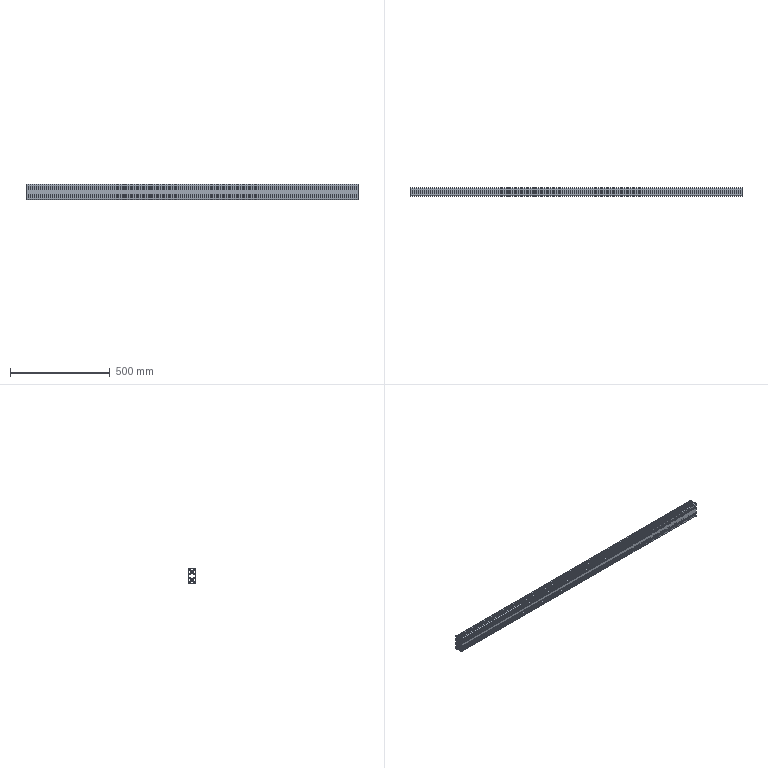Part | STEP file | MK-8-4080H-L-02 profile 4080H standard type 1620mm | 1 solid | 294 faces | box 1664 x 40 x 80 mm | volume 1350750 mm3 | cylinder 148 | plane 142 | cone 4 | commonest cylinder face diameters 0.6 x44 2 x44 4 x28 0.4 x14 6 x4 6.8 x4